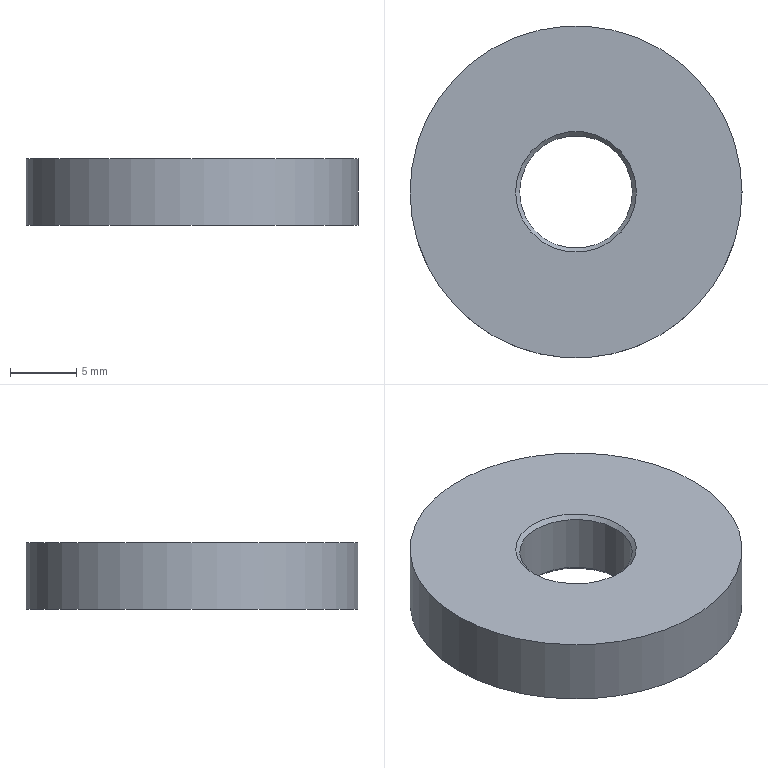Part | STEP file | 1 solid | 6 faces | box 25 x 25 x 5 mm | volume 2168 mm3 | plane 2 | cylinder 2 | cone 2 | commonest cylinder face diameters 8.5 x1 25 x1
STEP:
#1=CARTESIAN_POINT('',(0.,0.,0.));
#2=DIRECTION('',(0.,0.,1.));
#3=DIRECTION('',(1.,0.,0.));
#4=AXIS2_PLACEMENT_3D('',#1,#2,#3);
#5=CARTESIAN_POINT('',(1482.697,378.48,-85.381));
#6=VERTEX_POINT('',#5);
#7=CARTESIAN_POINT('',(1487.247,378.48,-85.381));
#8=DIRECTION('',(0.,0.,1.));
#9=DIRECTION('',(-1.,0.,0.));
#10=AXIS2_PLACEMENT_3D('',#7,#8,#9);
#11=CIRCLE('',#10,4.55);
#12=CARTESIAN_POINT('',(1487.247,378.48,-85.381));
#13=DIRECTION('',(0.,0.,-1.));
#14=DIRECTION('',(1.,0.,0.));
#15=AXIS2_PLACEMENT_3D('',#12,#13,#14);
#16=PLANE('',#15);
#17=CARTESIAN_POINT('',(-4.55,0.));
#18=CARTESIAN_POINT('',(-4.55,7.881));
#19=CARTESIAN_POINT('',(2.275,3.94));
#20=CARTESIAN_POINT('',(9.1,0.));
#21=CARTESIAN_POINT('',(2.275,-3.94));
#22=CARTESIAN_POINT('',(-4.55,-7.881));
#23=CARTESIAN_POINT('',(-4.55,0.));
#24=(BOUNDED_CURVE()B_SPLINE_CURVE(2,(#17,#18,#19,#20,#21,#22,#23),.UNSPECIFIED.,.T.,.F.)B_SPLINE_CURVE_WITH_KNOTS((1,2,2,2,2,1),(-2.094,0.,2.094,4.189,6.283,8.378),.UNSPECIFIED.)CURVE()GEOMETRIC_REPRESENTATION_ITEM()RATIONAL_B_SPLINE_CURVE((1.,0.5,1.,0.5,1.,0.5,1.))REPRESENTATION_ITEM(''));
#25=(GEOMETRIC_REPRESENTATION_CONTEXT(2)PARAMETRIC_REPRESENTATION_CONTEXT()REPRESENTATION_CONTEXT('',''));
#26=DEFINITIONAL_REPRESENTATION('',(#24),#25);
#27=PCURVE('',#16,#26);
#28=CARTESIAN_POINT('',(1487.247,378.48,-85.381));
#29=DIRECTION('',(0.,0.,-1.));
#30=DIRECTION('',(-1.,0.,0.));
#31=AXIS2_PLACEMENT_3D('',#28,#29,#30);
#32=CONICAL_SURFACE('',#31,4.55,0.7854);
#33=CARTESIAN_POINT('',(6.283,0.));
#34=DIRECTION('',(-1.,0.));
#35=VECTOR('',#34,1.);
#36=LINE('',#33,#35);
#37=(GEOMETRIC_REPRESENTATION_CONTEXT(2)PARAMETRIC_REPRESENTATION_CONTEXT()REPRESENTATION_CONTEXT('',''));
#38=DEFINITIONAL_REPRESENTATION('',(#36),#37);
#39=PCURVE('',#32,#38);
#40=SURFACE_CURVE('',#11,(#27,#39),.PCURVE_S1.);
#41=EDGE_CURVE('',#6,#6,#40,.T.);
#42=ORIENTED_EDGE('',*,*,#41,.T.);
#43=EDGE_LOOP('',(#42));
#44=FACE_BOUND('',#43,.T.);
#45=CARTESIAN_POINT('',(1474.747,378.48,-85.381));
#46=VERTEX_POINT('',#45);
#47=CARTESIAN_POINT('',(1487.247,378.48,-85.381));
#48=DIRECTION('',(0.,0.,1.));
#49=DIRECTION('',(-1.,0.,0.));
#50=AXIS2_PLACEMENT_3D('',#47,#48,#49);
#51=CIRCLE('',#50,12.5);
#52=CARTESIAN_POINT('',(-12.5,0.));
#53=CARTESIAN_POINT('',(-12.5,21.651));
#54=CARTESIAN_POINT('',(6.25,10.825));
#55=CARTESIAN_POINT('',(25.,0.));
#56=CARTESIAN_POINT('',(6.25,-10.825));
#57=CARTESIAN_POINT('',(-12.5,-21.651));
#58=CARTESIAN_POINT('',(-12.5,0.));
#59=(BOUNDED_CURVE()B_SPLINE_CURVE(2,(#52,#53,#54,#55,#56,#57,#58),.UNSPECIFIED.,.T.,.F.)B_SPLINE_CURVE_WITH_KNOTS((1,2,2,2,2,1),(-2.094,0.,2.094,4.189,6.283,8.378),.UNSPECIFIED.)CURVE()GEOMETRIC_REPRESENTATION_ITEM()RATIONAL_B_SPLINE_CURVE((1.,0.5,1.,0.5,1.,0.5,1.))REPRESENTATION_ITEM(''));
#60=(GEOMETRIC_REPRESENTATION_CONTEXT(2)PARAMETRIC_REPRESENTATION_CONTEXT()REPRESENTATION_CONTEXT('',''));
#61=DEFINITIONAL_REPRESENTATION('',(#59),#60);
#62=PCURVE('',#16,#61);
#63=CARTESIAN_POINT('',(1487.247,378.48,-83.381));
#64=DIRECTION('',(0.,0.,-1.));
#65=DIRECTION('',(-1.,0.,0.));
#66=AXIS2_PLACEMENT_3D('',#63,#64,#65);
#67=CYLINDRICAL_SURFACE('',#66,12.5);
#68=CARTESIAN_POINT('',(6.283,2.));
#69=DIRECTION('',(-1.,0.));
#70=VECTOR('',#69,1.);
#71=LINE('',#68,#70);
#72=(GEOMETRIC_REPRESENTATION_CONTEXT(2)PARAMETRIC_REPRESENTATION_CONTEXT()REPRESENTATION_CONTEXT('',''));
#73=DEFINITIONAL_REPRESENTATION('',(#71),#72);
#74=PCURVE('',#67,#73);
#75=SURFACE_CURVE('',#51,(#62,#74),.PCURVE_S1.);
#76=EDGE_CURVE('',#46,#46,#75,.T.);
#77=ORIENTED_EDGE('',*,*,#76,.F.);
#78=EDGE_LOOP('',(#77));
#79=FACE_BOUND('',#78,.T.);
#80=ADVANCED_FACE('',(#44,#79),#16,.T.);
#81=CARTESIAN_POINT('',(1499.747,378.48,-80.381));
#82=VERTEX_POINT('',#81);
#83=CARTESIAN_POINT('',(1474.747,378.48,-80.381));
#84=VERTEX_POINT('',#83);
#85=CARTESIAN_POINT('',(1487.247,378.48,-80.381));
#86=DIRECTION('',(0.,0.,-1.));
#87=DIRECTION('',(1.,0.,0.));
#88=AXIS2_PLACEMENT_3D('',#85,#86,#87);
#89=CIRCLE('',#88,12.5);
#90=CARTESIAN_POINT('',(3.142,-3.));
#91=DIRECTION('',(1.,0.));
#92=VECTOR('',#91,1.);
#93=LINE('',#90,#92);
#94=(GEOMETRIC_REPRESENTATION_CONTEXT(2)PARAMETRIC_REPRESENTATION_CONTEXT()REPRESENTATION_CONTEXT('',''));
#95=DEFINITIONAL_REPRESENTATION('',(#93),#94);
#96=PCURVE('',#67,#95);
#97=CARTESIAN_POINT('',(1487.247,378.48,-80.381));
#98=DIRECTION('',(0.,0.,1.));
#99=DIRECTION('',(-1.,0.,0.));
#100=AXIS2_PLACEMENT_3D('',#97,#98,#99);
#101=PLANE('',#100);
#102=CARTESIAN_POINT('',(-12.5,0.));
#103=CARTESIAN_POINT('',(-12.5,21.651));
#104=CARTESIAN_POINT('',(6.25,10.825));
#105=CARTESIAN_POINT('',(25.,0.));
#106=CARTESIAN_POINT('',(6.25,-10.825));
#107=CARTESIAN_POINT('',(-12.5,-21.651));
#108=CARTESIAN_POINT('',(-12.5,0.));
#109=(BOUNDED_CURVE()B_SPLINE_CURVE(2,(#102,#103,#104,#105,#106,#107,#108),.UNSPECIFIED.,.T.,.F.)B_SPLINE_CURVE_WITH_KNOTS((1,2,2,2,2,1),(-2.094,0.,2.094,4.189,6.283,8.378),.UNSPECIFIED.)CURVE()GEOMETRIC_REPRESENTATION_ITEM()RATIONAL_B_SPLINE_CURVE((1.,0.5,1.,0.5,1.,0.5,1.))REPRESENTATION_ITEM(''));
#110=(GEOMETRIC_REPRESENTATION_CONTEXT(2)PARAMETRIC_REPRESENTATION_CONTEXT()REPRESENTATION_CONTEXT('',''));
#111=DEFINITIONAL_REPRESENTATION('',(#109),#110);
#112=PCURVE('',#101,#111);
#113=SURFACE_CURVE('',#89,(#96,#112),.PCURVE_S1.);
#114=EDGE_CURVE('',#82,#84,#113,.T.);
#115=ORIENTED_EDGE('',*,*,#114,.T.);
#116=CARTESIAN_POINT('',(1474.747,378.48,-80.381));
#117=CARTESIAN_POINT('',(1474.747,378.48,-85.381));
#118=B_SPLINE_CURVE_WITH_KNOTS('',1,(#116,#117),.UNSPECIFIED.,.F.,.F.,(2,2),(-3.,2.),.PIECEWISE_BEZIER_KNOTS.);
#119=CARTESIAN_POINT('',(6.283,0.));
#120=DIRECTION('',(0.,1.));
#121=VECTOR('',#120,1.);
#122=LINE('',#119,#121);
#123=(GEOMETRIC_REPRESENTATION_CONTEXT(2)PARAMETRIC_REPRESENTATION_CONTEXT()REPRESENTATION_CONTEXT('',''));
#124=DEFINITIONAL_REPRESENTATION('',(#122),#123);
#125=PCURVE('',#67,#124);
#126=CARTESIAN_POINT('',(0.,0.));
#127=DIRECTION('',(0.,1.));
#128=VECTOR('',#127,1.);
#129=LINE('',#126,#128);
#130=(GEOMETRIC_REPRESENTATION_CONTEXT(2)PARAMETRIC_REPRESENTATION_CONTEXT()REPRESENTATION_CONTEXT('',''));
#131=DEFINITIONAL_REPRESENTATION('',(#129),#130);
#132=PCURVE('',#67,#131);
#133=SEAM_CURVE('',#118,(#125,#132),.PCURVE_S1.);
#134=EDGE_CURVE('',#84,#46,#133,.T.);
#135=ORIENTED_EDGE('',*,*,#134,.T.);
#136=ORIENTED_EDGE('',*,*,#76,.T.);
#137=ORIENTED_EDGE('',*,*,#134,.F.);
#138=CARTESIAN_POINT('',(1487.247,378.48,-80.381));
#139=DIRECTION('',(0.,0.,-1.));
#140=DIRECTION('',(1.,0.,0.));
#141=AXIS2_PLACEMENT_3D('',#138,#139,#140);
#142=CIRCLE('',#141,12.5);
#143=CARTESIAN_POINT('',(-3.142,-3.));
#144=DIRECTION('',(1.,0.));
#145=VECTOR('',#144,1.);
#146=LINE('',#143,#145);
#147=(GEOMETRIC_REPRESENTATION_CONTEXT(2)PARAMETRIC_REPRESENTATION_CONTEXT()REPRESENTATION_CONTEXT('',''));
#148=DEFINITIONAL_REPRESENTATION('',(#146),#147);
#149=PCURVE('',#67,#148);
#150=CARTESIAN_POINT('',(-12.5,0.));
#151=CARTESIAN_POINT('',(-12.5,21.651));
#152=CARTESIAN_POINT('',(6.25,10.825));
#153=CARTESIAN_POINT('',(25.,0.));
#154=CARTESIAN_POINT('',(6.25,-10.825));
#155=CARTESIAN_POINT('',(-12.5,-21.651));
#156=CARTESIAN_POINT('',(-12.5,0.));
#157=(BOUNDED_CURVE()B_SPLINE_CURVE(2,(#150,#151,#152,#153,#154,#155,#156),.UNSPECIFIED.,.T.,.F.)B_SPLINE_CURVE_WITH_KNOTS((1,2,2,2,2,1),(-2.094,0.,2.094,4.189,6.283,8.378),.UNSPECIFIED.)CURVE()GEOMETRIC_REPRESENTATION_ITEM()RATIONAL_B_SPLINE_CURVE((1.,0.5,1.,0.5,1.,0.5,1.))REPRESENTATION_ITEM(''));
#158=(GEOMETRIC_REPRESENTATION_CONTEXT(2)PARAMETRIC_REPRESENTATION_CONTEXT()REPRESENTATION_CONTEXT('',''));
#159=DEFINITIONAL_REPRESENTATION('',(#157),#158);
#160=PCURVE('',#101,#159);
#161=SURFACE_CURVE('',#142,(#149,#160),.PCURVE_S1.);
#162=EDGE_CURVE('',#84,#82,#161,.T.);
#163=ORIENTED_EDGE('',*,*,#162,.T.);
#164=EDGE_LOOP('',(#115,#135,#136,#137,#163));
#165=FACE_BOUND('',#164,.T.);
#166=ADVANCED_FACE('',(#165),#67,.T.);
#167=CARTESIAN_POINT('',(1482.997,378.48,-85.081));
#168=VERTEX_POINT('',#167);
#169=CARTESIAN_POINT('',(1487.247,378.48,-85.081));
#170=DIRECTION('',(0.,0.,-1.));
#171=DIRECTION('',(-1.,0.,0.));
#172=AXIS2_PLACEMENT_3D('',#169,#170,#171);
#173=CIRCLE('',#172,4.25);
#174=CARTESIAN_POINT('',(1487.247,378.48,-89.381));
#175=DIRECTION('',(0.,0.,1.));
#176=DIRECTION('',(-1.,0.,0.));
#177=AXIS2_PLACEMENT_3D('',#174,#175,#176);
#178=CYLINDRICAL_SURFACE('',#177,4.25);
#179=CARTESIAN_POINT('',(6.283,4.3));
#180=DIRECTION('',(-1.,0.));
#181=VECTOR('',#180,1.);
#182=LINE('',#179,#181);
#183=(GEOMETRIC_REPRESENTATION_CONTEXT(2)PARAMETRIC_REPRESENTATION_CONTEXT()REPRESENTATION_CONTEXT('',''));
#184=DEFINITIONAL_REPRESENTATION('',(#182),#183);
#185=PCURVE('',#178,#184);
#186=CARTESIAN_POINT('',(0.,-0.3));
#187=DIRECTION('',(1.,0.));
#188=VECTOR('',#187,1.);
#189=LINE('',#186,#188);
#190=(GEOMETRIC_REPRESENTATION_CONTEXT(2)PARAMETRIC_REPRESENTATION_CONTEXT()REPRESENTATION_CONTEXT('',''));
#191=DEFINITIONAL_REPRESENTATION('',(#189),#190);
#192=PCURVE('',#32,#191);
#193=SURFACE_CURVE('',#173,(#185,#192),.PCURVE_S1.);
#194=EDGE_CURVE('',#168,#168,#193,.T.);
#195=ORIENTED_EDGE('',*,*,#194,.F.);
#196=CARTESIAN_POINT('',(1482.997,378.48,-80.681));
#197=VERTEX_POINT('',#196);
#198=CARTESIAN_POINT('',(1482.997,378.48,-85.081));
#199=CARTESIAN_POINT('',(1482.997,378.48,-80.681));
#200=B_SPLINE_CURVE_WITH_KNOTS('',1,(#198,#199),.UNSPECIFIED.,.F.,.F.,(2,2),(4.3,8.7),.PIECEWISE_BEZIER_KNOTS.);
#201=CARTESIAN_POINT('',(6.283,0.));
#202=DIRECTION('',(0.,1.));
#203=VECTOR('',#202,1.);
#204=LINE('',#201,#203);
#205=(GEOMETRIC_REPRESENTATION_CONTEXT(2)PARAMETRIC_REPRESENTATION_CONTEXT()REPRESENTATION_CONTEXT('',''));
#206=DEFINITIONAL_REPRESENTATION('',(#204),#205);
#207=PCURVE('',#178,#206);
#208=CARTESIAN_POINT('',(0.,0.));
#209=DIRECTION('',(0.,1.));
#210=VECTOR('',#209,1.);
#211=LINE('',#208,#210);
#212=(GEOMETRIC_REPRESENTATION_CONTEXT(2)PARAMETRIC_REPRESENTATION_CONTEXT()REPRESENTATION_CONTEXT('',''));
#213=DEFINITIONAL_REPRESENTATION('',(#211),#212);
#214=PCURVE('',#178,#213);
#215=SEAM_CURVE('',#200,(#207,#214),.PCURVE_S1.);
#216=EDGE_CURVE('',#168,#197,#215,.T.);
#217=ORIENTED_EDGE('',*,*,#216,.T.);
#218=CARTESIAN_POINT('',(1491.497,378.48,-80.681));
#219=VERTEX_POINT('',#218);
#220=CARTESIAN_POINT('',(1487.247,378.48,-80.681));
#221=DIRECTION('',(0.,0.,1.));
#222=DIRECTION('',(1.,0.,0.));
#223=AXIS2_PLACEMENT_3D('',#220,#221,#222);
#224=CIRCLE('',#223,4.25);
#225=CARTESIAN_POINT('',(3.142,8.7));
#226=DIRECTION('',(1.,0.));
#227=VECTOR('',#226,1.);
#228=LINE('',#225,#227);
#229=(GEOMETRIC_REPRESENTATION_CONTEXT(2)PARAMETRIC_REPRESENTATION_CONTEXT()REPRESENTATION_CONTEXT('',''));
#230=DEFINITIONAL_REPRESENTATION('',(#228),#229);
#231=PCURVE('',#178,#230);
#232=CARTESIAN_POINT('',(1487.247,378.48,-80.381));
#233=DIRECTION('',(0.,0.,1.));
#234=DIRECTION('',(1.,0.,0.));
#235=AXIS2_PLACEMENT_3D('',#232,#233,#234);
#236=CONICAL_SURFACE('',#235,4.55,0.7854);
#237=CARTESIAN_POINT('',(0.,-0.3));
#238=DIRECTION('',(1.,0.));
#239=VECTOR('',#238,1.);
#240=LINE('',#237,#239);
#241=(GEOMETRIC_REPRESENTATION_CONTEXT(2)PARAMETRIC_REPRESENTATION_CONTEXT()REPRESENTATION_CONTEXT('',''));
#242=DEFINITIONAL_REPRESENTATION('',(#240),#241);
#243=PCURVE('',#236,#242);
#244=SURFACE_CURVE('',#224,(#231,#243),.PCURVE_S1.);
#245=EDGE_CURVE('',#219,#197,#244,.T.);
#246=ORIENTED_EDGE('',*,*,#245,.F.);
#247=CARTESIAN_POINT('',(1487.247,378.48,-80.681));
#248=DIRECTION('',(0.,0.,1.));
#249=DIRECTION('',(1.,0.,0.));
#250=AXIS2_PLACEMENT_3D('',#247,#248,#249);
#251=CIRCLE('',#250,4.25);
#252=CARTESIAN_POINT('',(-3.142,8.7));
#253=DIRECTION('',(1.,0.));
#254=VECTOR('',#253,1.);
#255=LINE('',#252,#254);
#256=(GEOMETRIC_REPRESENTATION_CONTEXT(2)PARAMETRIC_REPRESENTATION_CONTEXT()REPRESENTATION_CONTEXT('',''));
#257=DEFINITIONAL_REPRESENTATION('',(#255),#256);
#258=PCURVE('',#178,#257);
#259=CARTESIAN_POINT('',(0.,-0.3));
#260=DIRECTION('',(1.,0.));
#261=VECTOR('',#260,1.);
#262=LINE('',#259,#261);
#263=(GEOMETRIC_REPRESENTATION_CONTEXT(2)PARAMETRIC_REPRESENTATION_CONTEXT()REPRESENTATION_CONTEXT('',''));
#264=DEFINITIONAL_REPRESENTATION('',(#262),#263);
#265=PCURVE('',#236,#264);
#266=SURFACE_CURVE('',#251,(#258,#265),.PCURVE_S1.);
#267=EDGE_CURVE('',#197,#219,#266,.T.);
#268=ORIENTED_EDGE('',*,*,#267,.F.);
#269=ORIENTED_EDGE('',*,*,#216,.F.);
#270=EDGE_LOOP('',(#195,#217,#246,#268,#269));
#271=FACE_BOUND('',#270,.F.);
#272=ADVANCED_FACE('',(#271),#178,.F.);
#273=CARTESIAN_POINT('',(1491.797,378.48,-80.381));
#274=VERTEX_POINT('',#273);
#275=CARTESIAN_POINT('',(1487.247,378.48,-80.381));
#276=DIRECTION('',(0.,0.,-1.));
#277=DIRECTION('',(1.,0.,0.));
#278=AXIS2_PLACEMENT_3D('',#275,#276,#277);
#279=CIRCLE('',#278,4.55);
#280=CARTESIAN_POINT('',(-4.55,0.));
#281=CARTESIAN_POINT('',(-4.55,7.881));
#282=CARTESIAN_POINT('',(2.275,3.94));
#283=CARTESIAN_POINT('',(9.1,0.));
#284=CARTESIAN_POINT('',(2.275,-3.94));
#285=CARTESIAN_POINT('',(-4.55,-7.881));
#286=CARTESIAN_POINT('',(-4.55,0.));
#287=(BOUNDED_CURVE()B_SPLINE_CURVE(2,(#280,#281,#282,#283,#284,#285,#286),.UNSPECIFIED.,.T.,.F.)B_SPLINE_CURVE_WITH_KNOTS((1,2,2,2,2,1),(-2.094,0.,2.094,4.189,6.283,8.378),.UNSPECIFIED.)CURVE()GEOMETRIC_REPRESENTATION_ITEM()RATIONAL_B_SPLINE_CURVE((1.,0.5,1.,0.5,1.,0.5,1.))REPRESENTATION_ITEM(''));
#288=(GEOMETRIC_REPRESENTATION_CONTEXT(2)PARAMETRIC_REPRESENTATION_CONTEXT()REPRESENTATION_CONTEXT('',''));
#289=DEFINITIONAL_REPRESENTATION('',(#287),#288);
#290=PCURVE('',#101,#289);
#291=CARTESIAN_POINT('',(6.283,0.));
#292=DIRECTION('',(-1.,0.));
#293=VECTOR('',#292,1.);
#294=LINE('',#291,#293);
#295=(GEOMETRIC_REPRESENTATION_CONTEXT(2)PARAMETRIC_REPRESENTATION_CONTEXT()REPRESENTATION_CONTEXT('',''));
#296=DEFINITIONAL_REPRESENTATION('',(#294),#295);
#297=PCURVE('',#236,#296);
#298=SURFACE_CURVE('',#279,(#290,#297),.PCURVE_S1.);
#299=EDGE_CURVE('',#274,#274,#298,.T.);
#300=ORIENTED_EDGE('',*,*,#299,.T.);
#301=EDGE_LOOP('',(#300));
#302=FACE_BOUND('',#301,.T.);
#303=ORIENTED_EDGE('',*,*,#114,.F.);
#304=ORIENTED_EDGE('',*,*,#162,.F.);
#305=EDGE_LOOP('',(#303,#304));
#306=FACE_BOUND('',#305,.T.);
#307=ADVANCED_FACE('',(#302,#306),#101,.T.);
#308=ORIENTED_EDGE('',*,*,#194,.T.);
#309=CARTESIAN_POINT('',(1482.997,378.48,-85.081));
#310=CARTESIAN_POINT('',(1482.697,378.48,-85.381));
#311=B_SPLINE_CURVE_WITH_KNOTS('',1,(#309,#310),.UNSPECIFIED.,.F.,.F.,(2,2),(-0.4243,0.),.PIECEWISE_BEZIER_KNOTS.);
#312=CARTESIAN_POINT('',(6.283,0.));
#313=DIRECTION('',(0.,1.));
#314=VECTOR('',#313,1.);
#315=LINE('',#312,#314);
#316=(GEOMETRIC_REPRESENTATION_CONTEXT(2)PARAMETRIC_REPRESENTATION_CONTEXT()REPRESENTATION_CONTEXT('',''));
#317=DEFINITIONAL_REPRESENTATION('',(#315),#316);
#318=PCURVE('',#32,#317);
#319=CARTESIAN_POINT('',(0.,0.));
#320=DIRECTION('',(0.,1.));
#321=VECTOR('',#320,1.);
#322=LINE('',#319,#321);
#323=(GEOMETRIC_REPRESENTATION_CONTEXT(2)PARAMETRIC_REPRESENTATION_CONTEXT()REPRESENTATION_CONTEXT('',''));
#324=DEFINITIONAL_REPRESENTATION('',(#322),#323);
#325=PCURVE('',#32,#324);
#326=SEAM_CURVE('',#311,(#318,#325),.PCURVE_S1.);
#327=EDGE_CURVE('',#168,#6,#326,.T.);
#328=ORIENTED_EDGE('',*,*,#327,.T.);
#329=ORIENTED_EDGE('',*,*,#41,.T.);
#330=ORIENTED_EDGE('',*,*,#327,.F.);
#331=EDGE_LOOP('',(#308,#328,#329,#330));
#332=FACE_BOUND('',#331,.F.);
#333=ADVANCED_FACE('',(#332),#32,.F.);
#334=ORIENTED_EDGE('',*,*,#267,.T.);
#335=CARTESIAN_POINT('',(1491.497,378.48,-80.681));
#336=CARTESIAN_POINT('',(1491.797,378.48,-80.381));
#337=B_SPLINE_CURVE_WITH_KNOTS('',1,(#335,#336),.UNSPECIFIED.,.F.,.F.,(2,2),(-0.4243,0.),.PIECEWISE_BEZIER_KNOTS.);
#338=CARTESIAN_POINT('',(6.283,0.));
#339=DIRECTION('',(0.,1.));
#340=VECTOR('',#339,1.);
#341=LINE('',#338,#340);
#342=(GEOMETRIC_REPRESENTATION_CONTEXT(2)PARAMETRIC_REPRESENTATION_CONTEXT()REPRESENTATION_CONTEXT('',''));
#343=DEFINITIONAL_REPRESENTATION('',(#341),#342);
#344=PCURVE('',#236,#343);
#345=CARTESIAN_POINT('',(0.,0.));
#346=DIRECTION('',(0.,1.));
#347=VECTOR('',#346,1.);
#348=LINE('',#345,#347);
#349=(GEOMETRIC_REPRESENTATION_CONTEXT(2)PARAMETRIC_REPRESENTATION_CONTEXT()REPRESENTATION_CONTEXT('',''));
#350=DEFINITIONAL_REPRESENTATION('',(#348),#349);
#351=PCURVE('',#236,#350);
#352=SEAM_CURVE('',#337,(#344,#351),.PCURVE_S1.);
#353=EDGE_CURVE('',#219,#274,#352,.T.);
#354=ORIENTED_EDGE('',*,*,#353,.T.);
#355=ORIENTED_EDGE('',*,*,#299,.T.);
#356=ORIENTED_EDGE('',*,*,#353,.F.);
#357=ORIENTED_EDGE('',*,*,#245,.T.);
#358=EDGE_LOOP('',(#334,#354,#355,#356,#357));
#359=FACE_BOUND('',#358,.F.);
#360=ADVANCED_FACE('',(#359),#236,.F.);
#361=CLOSED_SHELL('',(#80,#166,#272,#307,#333,#360));
#362=MANIFOLD_SOLID_BREP('',#361);
#363=(LENGTH_UNIT()NAMED_UNIT(*)SI_UNIT(.MILLI.,.METRE.));
#364=UNCERTAINTY_MEASURE_WITH_UNIT(LENGTH_MEASURE(0.00001),#363,'','');
#365=(NAMED_UNIT(*)PLANE_ANGLE_UNIT()SI_UNIT($,.RADIAN.));
#366=(NAMED_UNIT(*)SI_UNIT($,.STERADIAN.)SOLID_ANGLE_UNIT());
#367=(GEOMETRIC_REPRESENTATION_CONTEXT(3)GLOBAL_UNCERTAINTY_ASSIGNED_CONTEXT((#364))GLOBAL_UNIT_ASSIGNED_CONTEXT((#363,#365,#366))REPRESENTATION_CONTEXT('',''));
#368=ADVANCED_BREP_SHAPE_REPRESENTATION('',(#4,#362),#367);